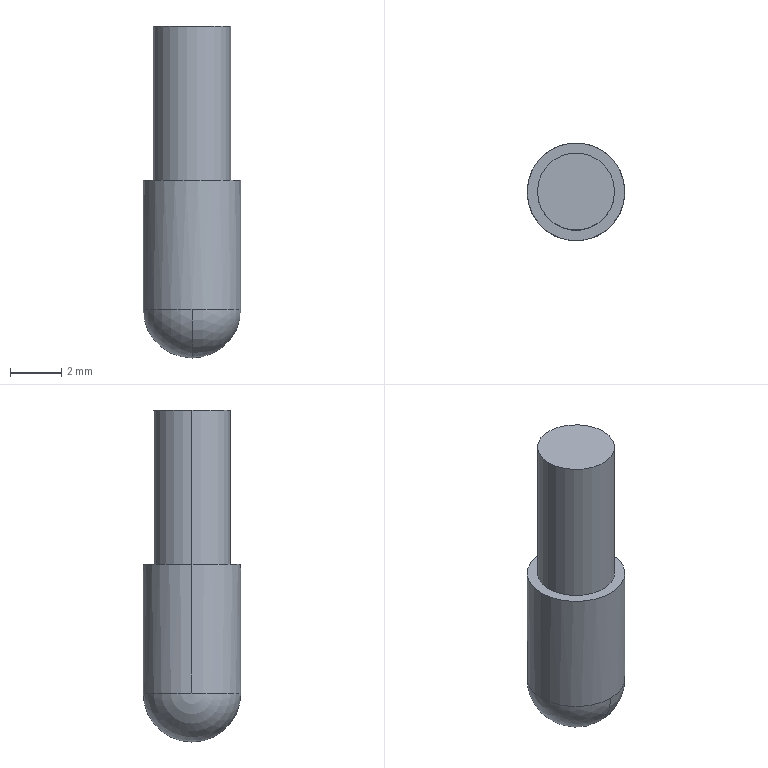Part | STEP file | CKFQAGG3-P3.8-L6-B5_Default | 1 solid | 8 faces | box 3.8 x 3.8 x 12.9 mm | volume 113.483 mm3 | cylinder 4 | sphere 2 | plane 2 | commonest cylinder face diameters 3 x2 3.8 x2
STEP:
#1=CARTESIAN_POINT('',(0.,0.,0.));
#2=DIRECTION('',(0.,0.,1.));
#3=DIRECTION('',(1.,0.,0.));
#4=AXIS2_PLACEMENT_3D('',#1,#2,#3);
#5=CARTESIAN_POINT('',(-1.5,0.,12.9));
#6=VERTEX_POINT('',#5);
#7=CARTESIAN_POINT('',(1.5,0.,12.9));
#8=VERTEX_POINT('',#7);
#9=CARTESIAN_POINT('',(0.,0.,12.9));
#10=DIRECTION('',(0.,0.,-1.));
#11=DIRECTION('',(-1.,0.,0.));
#12=AXIS2_PLACEMENT_3D('',#9,#10,#11);
#13=CIRCLE('',#12,1.5);
#14=CARTESIAN_POINT('',(0.,0.,0.));
#15=DIRECTION('',(0.,0.,-1.));
#16=DIRECTION('',(-1.,0.,0.));
#17=AXIS2_PLACEMENT_3D('',#14,#15,#16);
#18=CYLINDRICAL_SURFACE('',#17,1.5);
#19=CARTESIAN_POINT('',(0.,-12.9));
#20=DIRECTION('',(1.,0.));
#21=VECTOR('',#20,1.);
#22=LINE('',#19,#21);
#23=(GEOMETRIC_REPRESENTATION_CONTEXT(2)PARAMETRIC_REPRESENTATION_CONTEXT()REPRESENTATION_CONTEXT('',''));
#24=DEFINITIONAL_REPRESENTATION('',(#22),#23);
#25=PCURVE('',#18,#24);
#26=CARTESIAN_POINT('',(0.,1.5,12.9));
#27=DIRECTION('',(0.,0.,1.));
#28=DIRECTION('',(1.,0.,0.));
#29=AXIS2_PLACEMENT_3D('',#26,#27,#28);
#30=PLANE('',#29);
#31=CARTESIAN_POINT('',(-1.5,-1.5));
#32=CARTESIAN_POINT('',(-1.5,1.098));
#33=CARTESIAN_POINT('',(0.75,-0.201));
#34=CARTESIAN_POINT('',(3.,-1.5));
#35=CARTESIAN_POINT('',(0.75,-2.799));
#36=CARTESIAN_POINT('',(-1.5,-4.098));
#37=CARTESIAN_POINT('',(-1.5,-1.5));
#38=(BOUNDED_CURVE()B_SPLINE_CURVE(2,(#31,#32,#33,#34,#35,#36,#37),.UNSPECIFIED.,.T.,.F.)B_SPLINE_CURVE_WITH_KNOTS((1,2,2,2,2,1),(-2.094,0.,2.094,4.189,6.283,8.378),.UNSPECIFIED.)CURVE()GEOMETRIC_REPRESENTATION_ITEM()RATIONAL_B_SPLINE_CURVE((1.,0.5,1.,0.5,1.,0.5,1.))REPRESENTATION_ITEM(''));
#39=(GEOMETRIC_REPRESENTATION_CONTEXT(2)PARAMETRIC_REPRESENTATION_CONTEXT()REPRESENTATION_CONTEXT('',''));
#40=DEFINITIONAL_REPRESENTATION('',(#38),#39);
#41=PCURVE('',#30,#40);
#42=SURFACE_CURVE('',#13,(#25,#41),.PCURVE_S1.);
#43=EDGE_CURVE('',#6,#8,#42,.T.);
#44=ORIENTED_EDGE('',*,*,#43,.T.);
#45=CARTESIAN_POINT('',(1.5,0.,6.9));
#46=VERTEX_POINT('',#45);
#47=CARTESIAN_POINT('',(1.5,0.,0.));
#48=DIRECTION('',(0.,0.,-1.));
#49=VECTOR('',#48,1.);
#50=LINE('',#47,#49);
#51=CARTESIAN_POINT('',(3.142,0.));
#52=DIRECTION('',(0.,1.));
#53=VECTOR('',#52,1.);
#54=LINE('',#51,#53);
#55=(GEOMETRIC_REPRESENTATION_CONTEXT(2)PARAMETRIC_REPRESENTATION_CONTEXT()REPRESENTATION_CONTEXT('',''));
#56=DEFINITIONAL_REPRESENTATION('',(#54),#55);
#57=PCURVE('',#18,#56);
#58=CARTESIAN_POINT('',(0.,0.,0.));
#59=DIRECTION('',(0.,0.,-1.));
#60=DIRECTION('',(-1.,0.,0.));
#61=AXIS2_PLACEMENT_3D('',#58,#59,#60);
#62=CYLINDRICAL_SURFACE('',#61,1.5);
#63=CARTESIAN_POINT('',(3.142,0.));
#64=DIRECTION('',(0.,1.));
#65=VECTOR('',#64,1.);
#66=LINE('',#63,#65);
#67=(GEOMETRIC_REPRESENTATION_CONTEXT(2)PARAMETRIC_REPRESENTATION_CONTEXT()REPRESENTATION_CONTEXT('',''));
#68=DEFINITIONAL_REPRESENTATION('',(#66),#67);
#69=PCURVE('',#62,#68);
#70=SURFACE_CURVE('',#50,(#57,#69),.PCURVE_S1.);
#71=EDGE_CURVE('',#8,#46,#70,.T.);
#72=ORIENTED_EDGE('',*,*,#71,.T.);
#73=CARTESIAN_POINT('',(-1.5,0.,6.9));
#74=VERTEX_POINT('',#73);
#75=CARTESIAN_POINT('',(0.,0.,6.9));
#76=DIRECTION('',(0.,0.,-1.));
#77=DIRECTION('',(-1.,0.,0.));
#78=AXIS2_PLACEMENT_3D('',#75,#76,#77);
#79=CIRCLE('',#78,1.5);
#80=CARTESIAN_POINT('',(0.,-6.9));
#81=DIRECTION('',(1.,0.));
#82=VECTOR('',#81,1.);
#83=LINE('',#80,#82);
#84=(GEOMETRIC_REPRESENTATION_CONTEXT(2)PARAMETRIC_REPRESENTATION_CONTEXT()REPRESENTATION_CONTEXT('',''));
#85=DEFINITIONAL_REPRESENTATION('',(#83),#84);
#86=PCURVE('',#18,#85);
#87=CARTESIAN_POINT('',(0.,1.9,6.9));
#88=DIRECTION('',(0.,0.,1.));
#89=DIRECTION('',(1.,0.,0.));
#90=AXIS2_PLACEMENT_3D('',#87,#88,#89);
#91=PLANE('',#90);
#92=CARTESIAN_POINT('',(-1.5,-1.9));
#93=CARTESIAN_POINT('',(-1.5,0.6981));
#94=CARTESIAN_POINT('',(0.75,-0.601));
#95=CARTESIAN_POINT('',(3.,-1.9));
#96=CARTESIAN_POINT('',(0.75,-3.199));
#97=CARTESIAN_POINT('',(-1.5,-4.498));
#98=CARTESIAN_POINT('',(-1.5,-1.9));
#99=(BOUNDED_CURVE()B_SPLINE_CURVE(2,(#92,#93,#94,#95,#96,#97,#98),.UNSPECIFIED.,.T.,.F.)B_SPLINE_CURVE_WITH_KNOTS((1,2,2,2,2,1),(-2.094,0.,2.094,4.189,6.283,8.378),.UNSPECIFIED.)CURVE()GEOMETRIC_REPRESENTATION_ITEM()RATIONAL_B_SPLINE_CURVE((1.,0.5,1.,0.5,1.,0.5,1.))REPRESENTATION_ITEM(''));
#100=(GEOMETRIC_REPRESENTATION_CONTEXT(2)PARAMETRIC_REPRESENTATION_CONTEXT()REPRESENTATION_CONTEXT('',''));
#101=DEFINITIONAL_REPRESENTATION('',(#99),#100);
#102=PCURVE('',#91,#101);
#103=SURFACE_CURVE('',#79,(#86,#102),.PCURVE_S1.);
#104=EDGE_CURVE('',#74,#46,#103,.T.);
#105=ORIENTED_EDGE('',*,*,#104,.F.);
#106=CARTESIAN_POINT('',(-1.5,0.,0.));
#107=DIRECTION('',(0.,0.,-1.));
#108=VECTOR('',#107,1.);
#109=LINE('',#106,#108);
#110=CARTESIAN_POINT('',(0.,0.));
#111=DIRECTION('',(0.,1.));
#112=VECTOR('',#111,1.);
#113=LINE('',#110,#112);
#114=(GEOMETRIC_REPRESENTATION_CONTEXT(2)PARAMETRIC_REPRESENTATION_CONTEXT()REPRESENTATION_CONTEXT('',''));
#115=DEFINITIONAL_REPRESENTATION('',(#113),#114);
#116=PCURVE('',#18,#115);
#117=CARTESIAN_POINT('',(6.283,0.));
#118=DIRECTION('',(0.,1.));
#119=VECTOR('',#118,1.);
#120=LINE('',#117,#119);
#121=(GEOMETRIC_REPRESENTATION_CONTEXT(2)PARAMETRIC_REPRESENTATION_CONTEXT()REPRESENTATION_CONTEXT('',''));
#122=DEFINITIONAL_REPRESENTATION('',(#120),#121);
#123=PCURVE('',#62,#122);
#124=SURFACE_CURVE('',#109,(#116,#123),.PCURVE_S1.);
#125=EDGE_CURVE('',#6,#74,#124,.T.);
#126=ORIENTED_EDGE('',*,*,#125,.F.);
#127=EDGE_LOOP('',(#44,#72,#105,#126));
#128=FACE_BOUND('',#127,.T.);
#129=ADVANCED_FACE('',(#128),#18,.T.);
#130=CARTESIAN_POINT('',(-1.9,0.,6.9));
#131=VERTEX_POINT('',#130);
#132=CARTESIAN_POINT('',(1.9,0.,6.9));
#133=VERTEX_POINT('',#132);
#134=CARTESIAN_POINT('',(0.,0.,6.9));
#135=DIRECTION('',(0.,0.,-1.));
#136=DIRECTION('',(-1.,0.,0.));
#137=AXIS2_PLACEMENT_3D('',#134,#135,#136);
#138=CIRCLE('',#137,1.9);
#139=CARTESIAN_POINT('',(0.,0.,0.));
#140=DIRECTION('',(0.,0.,-1.));
#141=DIRECTION('',(-1.,0.,0.));
#142=AXIS2_PLACEMENT_3D('',#139,#140,#141);
#143=CYLINDRICAL_SURFACE('',#142,1.9);
#144=CARTESIAN_POINT('',(0.,-6.9));
#145=DIRECTION('',(1.,0.));
#146=VECTOR('',#145,1.);
#147=LINE('',#144,#146);
#148=(GEOMETRIC_REPRESENTATION_CONTEXT(2)PARAMETRIC_REPRESENTATION_CONTEXT()REPRESENTATION_CONTEXT('',''));
#149=DEFINITIONAL_REPRESENTATION('',(#147),#148);
#150=PCURVE('',#143,#149);
#151=CARTESIAN_POINT('',(-1.9,-1.9));
#152=CARTESIAN_POINT('',(-1.9,1.391));
#153=CARTESIAN_POINT('',(0.95,-0.2546));
#154=CARTESIAN_POINT('',(3.8,-1.9));
#155=CARTESIAN_POINT('',(0.95,-3.545));
#156=CARTESIAN_POINT('',(-1.9,-5.191));
#157=CARTESIAN_POINT('',(-1.9,-1.9));
#158=(BOUNDED_CURVE()B_SPLINE_CURVE(2,(#151,#152,#153,#154,#155,#156,#157),.UNSPECIFIED.,.T.,.F.)B_SPLINE_CURVE_WITH_KNOTS((1,2,2,2,2,1),(-2.094,0.,2.094,4.189,6.283,8.378),.UNSPECIFIED.)CURVE()GEOMETRIC_REPRESENTATION_ITEM()RATIONAL_B_SPLINE_CURVE((1.,0.5,1.,0.5,1.,0.5,1.))REPRESENTATION_ITEM(''));
#159=(GEOMETRIC_REPRESENTATION_CONTEXT(2)PARAMETRIC_REPRESENTATION_CONTEXT()REPRESENTATION_CONTEXT('',''));
#160=DEFINITIONAL_REPRESENTATION('',(#158),#159);
#161=PCURVE('',#91,#160);
#162=SURFACE_CURVE('',#138,(#150,#161),.PCURVE_S1.);
#163=EDGE_CURVE('',#131,#133,#162,.T.);
#164=ORIENTED_EDGE('',*,*,#163,.T.);
#165=CARTESIAN_POINT('',(1.9,0.,1.9));
#166=VERTEX_POINT('',#165);
#167=CARTESIAN_POINT('',(1.9,0.,0.));
#168=DIRECTION('',(0.,0.,-1.));
#169=VECTOR('',#168,1.);
#170=LINE('',#167,#169);
#171=CARTESIAN_POINT('',(3.142,0.));
#172=DIRECTION('',(0.,1.));
#173=VECTOR('',#172,1.);
#174=LINE('',#171,#173);
#175=(GEOMETRIC_REPRESENTATION_CONTEXT(2)PARAMETRIC_REPRESENTATION_CONTEXT()REPRESENTATION_CONTEXT('',''));
#176=DEFINITIONAL_REPRESENTATION('',(#174),#175);
#177=PCURVE('',#143,#176);
#178=CARTESIAN_POINT('',(0.,0.,0.));
#179=DIRECTION('',(0.,0.,-1.));
#180=DIRECTION('',(-1.,0.,0.));
#181=AXIS2_PLACEMENT_3D('',#178,#179,#180);
#182=CYLINDRICAL_SURFACE('',#181,1.9);
#183=CARTESIAN_POINT('',(3.142,0.));
#184=DIRECTION('',(0.,1.));
#185=VECTOR('',#184,1.);
#186=LINE('',#183,#185);
#187=(GEOMETRIC_REPRESENTATION_CONTEXT(2)PARAMETRIC_REPRESENTATION_CONTEXT()REPRESENTATION_CONTEXT('',''));
#188=DEFINITIONAL_REPRESENTATION('',(#186),#187);
#189=PCURVE('',#182,#188);
#190=SURFACE_CURVE('',#170,(#177,#189),.PCURVE_S1.);
#191=EDGE_CURVE('',#133,#166,#190,.T.);
#192=ORIENTED_EDGE('',*,*,#191,.T.);
#193=CARTESIAN_POINT('',(0.,1.9,1.9));
#194=VERTEX_POINT('',#193);
#195=CARTESIAN_POINT('',(0.,0.,1.9));
#196=DIRECTION('',(0.,0.,-1.));
#197=DIRECTION('',(-1.,0.,0.));
#198=AXIS2_PLACEMENT_3D('',#195,#196,#197);
#199=CIRCLE('',#198,1.9);
#200=CARTESIAN_POINT('',(0.,-1.9));
#201=DIRECTION('',(1.,0.));
#202=VECTOR('',#201,1.);
#203=LINE('',#200,#202);
#204=(GEOMETRIC_REPRESENTATION_CONTEXT(2)PARAMETRIC_REPRESENTATION_CONTEXT()REPRESENTATION_CONTEXT('',''));
#205=DEFINITIONAL_REPRESENTATION('',(#203),#204);
#206=PCURVE('',#143,#205);
#207=CARTESIAN_POINT('',(0.,0.,1.9));
#208=DIRECTION('',(-1.,0.,0.));
#209=DIRECTION('',(0.,-1.,0.));
#210=AXIS2_PLACEMENT_3D('',#207,#208,#209);
#211=SPHERICAL_SURFACE('',#210,1.9);
#212=CARTESIAN_POINT('',(3.142,1.571));
#213=DIRECTION('',(0.,-1.));
#214=VECTOR('',#213,1.);
#215=LINE('',#212,#214);
#216=(GEOMETRIC_REPRESENTATION_CONTEXT(2)PARAMETRIC_REPRESENTATION_CONTEXT()REPRESENTATION_CONTEXT('',''));
#217=DEFINITIONAL_REPRESENTATION('',(#215),#216);
#218=PCURVE('',#211,#217);
#219=SURFACE_CURVE('',#199,(#206,#218),.PCURVE_S1.);
#220=EDGE_CURVE('',#194,#166,#219,.T.);
#221=ORIENTED_EDGE('',*,*,#220,.F.);
#222=CARTESIAN_POINT('',(-1.9,0.,1.9));
#223=VERTEX_POINT('',#222);
#224=CARTESIAN_POINT('',(0.,0.,1.9));
#225=DIRECTION('',(0.,0.,-1.));
#226=DIRECTION('',(-1.,0.,0.));
#227=AXIS2_PLACEMENT_3D('',#224,#225,#226);
#228=CIRCLE('',#227,1.9);
#229=CARTESIAN_POINT('',(0.,-1.9));
#230=DIRECTION('',(1.,0.));
#231=VECTOR('',#230,1.);
#232=LINE('',#229,#231);
#233=(GEOMETRIC_REPRESENTATION_CONTEXT(2)PARAMETRIC_REPRESENTATION_CONTEXT()REPRESENTATION_CONTEXT('',''));
#234=DEFINITIONAL_REPRESENTATION('',(#232),#233);
#235=PCURVE('',#143,#234);
#236=CARTESIAN_POINT('',(0.,0.,1.9));
#237=DIRECTION('',(-1.,0.,0.));
#238=DIRECTION('',(0.,-1.,0.));
#239=AXIS2_PLACEMENT_3D('',#236,#237,#238);
#240=SPHERICAL_SURFACE('',#239,1.9);
#241=CARTESIAN_POINT('',(3.142,1.571));
#242=CARTESIAN_POINT('',(3.142,1.547));
#243=CARTESIAN_POINT('',(3.142,1.499));
#244=CARTESIAN_POINT('',(3.142,1.428));
#245=CARTESIAN_POINT('',(3.142,1.357));
#246=CARTESIAN_POINT('',(3.142,1.285));
#247=CARTESIAN_POINT('',(3.142,1.214));
#248=CARTESIAN_POINT('',(3.142,1.142));
#249=CARTESIAN_POINT('',(3.142,1.071));
#250=CARTESIAN_POINT('',(3.142,0.9996));
#251=CARTESIAN_POINT('',(3.142,0.9282));
#252=CARTESIAN_POINT('',(3.142,0.8568));
#253=CARTESIAN_POINT('',(3.142,0.7854));
#254=CARTESIAN_POINT('',(3.142,0.714));
#255=CARTESIAN_POINT('',(3.142,0.6426));
#256=CARTESIAN_POINT('',(3.142,0.5712));
#257=CARTESIAN_POINT('',(3.142,0.4998));
#258=CARTESIAN_POINT('',(3.142,0.4284));
#259=CARTESIAN_POINT('',(3.142,0.357));
#260=CARTESIAN_POINT('',(3.142,0.2856));
#261=CARTESIAN_POINT('',(3.142,0.2142));
#262=CARTESIAN_POINT('',(3.142,0.1428));
#263=CARTESIAN_POINT('',(3.142,0.0714));
#264=CARTESIAN_POINT('',(3.142,0.0238));
#265=CARTESIAN_POINT('',(3.142,0.));
#266=B_SPLINE_CURVE_WITH_KNOTS('',3,(#241,#242,#243,#244,#245,#246,#247,#248,#249,#250,#251,#252,#253,#254,#255,#256,#257,#258,#259,#260,#261,#262,#263,#264,#265),.UNSPECIFIED.,.F.,.F.,(4,1,1,1,1,1,1,1,1,1,1,1,1,1,1,1,1,1,1,1,1,1,4),(0.,0.0714,0.1428,0.2142,0.2856,0.357,0.4284,0.4998,0.5712,0.6426,0.714,0.7854,0.8568,0.9282,0.9996,1.071,1.142,1.214,1.285,1.357,1.428,1.499,1.571),.QUASI_UNIFORM_KNOTS.);
#267=(GEOMETRIC_REPRESENTATION_CONTEXT(2)PARAMETRIC_REPRESENTATION_CONTEXT()REPRESENTATION_CONTEXT('',''));
#268=DEFINITIONAL_REPRESENTATION('',(#266),#267);
#269=PCURVE('',#240,#268);
#270=SURFACE_CURVE('',#228,(#235,#269),.PCURVE_S1.);
#271=EDGE_CURVE('',#223,#194,#270,.T.);
#272=ORIENTED_EDGE('',*,*,#271,.F.);
#273=CARTESIAN_POINT('',(-1.9,0.,0.));
#274=DIRECTION('',(0.,0.,-1.));
#275=VECTOR('',#274,1.);
#276=LINE('',#273,#275);
#277=CARTESIAN_POINT('',(0.,0.));
#278=DIRECTION('',(0.,1.));
#279=VECTOR('',#278,1.);
#280=LINE('',#277,#279);
#281=(GEOMETRIC_REPRESENTATION_CONTEXT(2)PARAMETRIC_REPRESENTATION_CONTEXT()REPRESENTATION_CONTEXT('',''));
#282=DEFINITIONAL_REPRESENTATION('',(#280),#281);
#283=PCURVE('',#143,#282);
#284=CARTESIAN_POINT('',(6.283,0.));
#285=DIRECTION('',(0.,1.));
#286=VECTOR('',#285,1.);
#287=LINE('',#284,#286);
#288=(GEOMETRIC_REPRESENTATION_CONTEXT(2)PARAMETRIC_REPRESENTATION_CONTEXT()REPRESENTATION_CONTEXT('',''));
#289=DEFINITIONAL_REPRESENTATION('',(#287),#288);
#290=PCURVE('',#182,#289);
#291=SURFACE_CURVE('',#276,(#283,#290),.PCURVE_S1.);
#292=EDGE_CURVE('',#131,#223,#291,.T.);
#293=ORIENTED_EDGE('',*,*,#292,.F.);
#294=EDGE_LOOP('',(#164,#192,#221,#272,#293));
#295=FACE_BOUND('',#294,.T.);
#296=ADVANCED_FACE('',(#295),#143,.T.);
#297=CARTESIAN_POINT('',(0.,-1.9,1.9));
#298=VERTEX_POINT('',#297);
#299=CARTESIAN_POINT('',(0.,0.,1.9));
#300=DIRECTION('',(0.,0.,-1.));
#301=DIRECTION('',(-1.,0.,0.));
#302=AXIS2_PLACEMENT_3D('',#299,#300,#301);
#303=CIRCLE('',#302,1.9);
#304=CARTESIAN_POINT('',(6.283,-4.712));
#305=DIRECTION('',(0.,1.));
#306=VECTOR('',#305,1.);
#307=LINE('',#304,#306);
#308=(GEOMETRIC_REPRESENTATION_CONTEXT(2)PARAMETRIC_REPRESENTATION_CONTEXT()REPRESENTATION_CONTEXT('',''));
#309=DEFINITIONAL_REPRESENTATION('',(#307),#308);
#310=PCURVE('',#240,#309);
#311=CARTESIAN_POINT('',(0.,-1.9));
#312=DIRECTION('',(1.,0.));
#313=VECTOR('',#312,1.);
#314=LINE('',#311,#313);
#315=(GEOMETRIC_REPRESENTATION_CONTEXT(2)PARAMETRIC_REPRESENTATION_CONTEXT()REPRESENTATION_CONTEXT('',''));
#316=DEFINITIONAL_REPRESENTATION('',(#314),#315);
#317=PCURVE('',#182,#316);
#318=SURFACE_CURVE('',#303,(#310,#317),.PCURVE_S1.);
#319=EDGE_CURVE('',#298,#223,#318,.T.);
#320=ORIENTED_EDGE('',*,*,#319,.T.);
#321=ORIENTED_EDGE('',*,*,#271,.T.);
#322=CARTESIAN_POINT('',(0.,0.,0.));
#323=VERTEX_POINT('',#322);
#324=CARTESIAN_POINT('',(0.,0.,1.9));
#325=DIRECTION('',(-1.,0.,0.));
#326=DIRECTION('',(0.,-1.,0.));
#327=AXIS2_PLACEMENT_3D('',#324,#325,#326);
#328=CIRCLE('',#327,1.9);
#329=CARTESIAN_POINT('',(0.,0.));
#330=DIRECTION('',(1.,0.));
#331=VECTOR('',#330,1.);
#332=LINE('',#329,#331);
#333=(GEOMETRIC_REPRESENTATION_CONTEXT(2)PARAMETRIC_REPRESENTATION_CONTEXT()REPRESENTATION_CONTEXT('',''));
#334=DEFINITIONAL_REPRESENTATION('',(#332),#333);
#335=PCURVE('',#240,#334);
#336=CARTESIAN_POINT('',(0.,0.));
#337=DIRECTION('',(1.,0.));
#338=VECTOR('',#337,1.);
#339=LINE('',#336,#338);
#340=(GEOMETRIC_REPRESENTATION_CONTEXT(2)PARAMETRIC_REPRESENTATION_CONTEXT()REPRESENTATION_CONTEXT('',''));
#341=DEFINITIONAL_REPRESENTATION('',(#339),#340);
#342=PCURVE('',#211,#341);
#343=SURFACE_CURVE('',#328,(#335,#342),.PCURVE_S1.);
#344=EDGE_CURVE('',#194,#323,#343,.T.);
#345=ORIENTED_EDGE('',*,*,#344,.T.);
#346=CARTESIAN_POINT('',(0.,0.,1.9));
#347=DIRECTION('',(1.,0.,0.));
#348=DIRECTION('',(0.,0.,-1.));
#349=AXIS2_PLACEMENT_3D('',#346,#347,#348);
#350=CIRCLE('',#349,1.9);
#351=CARTESIAN_POINT('',(6.283,0.));
#352=CARTESIAN_POINT('',(6.259,0.));
#353=CARTESIAN_POINT('',(6.212,0.));
#354=CARTESIAN_POINT('',(6.14,0.));
#355=CARTESIAN_POINT('',(6.069,0.));
#356=CARTESIAN_POINT('',(5.998,0.));
#357=CARTESIAN_POINT('',(5.926,0.));
#358=CARTESIAN_POINT('',(5.855,0.));
#359=CARTESIAN_POINT('',(5.783,0.));
#360=CARTESIAN_POINT('',(5.712,0.));
#361=CARTESIAN_POINT('',(5.641,0.));
#362=CARTESIAN_POINT('',(5.569,0.));
#363=CARTESIAN_POINT('',(5.498,0.));
#364=CARTESIAN_POINT('',(5.426,0.));
#365=CARTESIAN_POINT('',(5.355,0.));
#366=CARTESIAN_POINT('',(5.284,0.));
#367=CARTESIAN_POINT('',(5.212,0.));
#368=CARTESIAN_POINT('',(5.141,0.));
#369=CARTESIAN_POINT('',(5.069,0.));
#370=CARTESIAN_POINT('',(4.998,0.));
#371=CARTESIAN_POINT('',(4.927,0.));
#372=CARTESIAN_POINT('',(4.855,0.));
#373=CARTESIAN_POINT('',(4.784,0.));
#374=CARTESIAN_POINT('',(4.736,0.));
#375=CARTESIAN_POINT('',(4.712,0.));
#376=B_SPLINE_CURVE_WITH_KNOTS('',3,(#351,#352,#353,#354,#355,#356,#357,#358,#359,#360,#361,#362,#363,#364,#365,#366,#367,#368,#369,#370,#371,#372,#373,#374,#375),.UNSPECIFIED.,.F.,.F.,(4,1,1,1,1,1,1,1,1,1,1,1,1,1,1,1,1,1,1,1,1,1,4),(4.712,4.784,4.855,4.927,4.998,5.069,5.141,5.212,5.284,5.355,5.426,5.498,5.569,5.641,5.712,5.783,5.855,5.926,5.998,6.069,6.14,6.212,6.283),.QUASI_UNIFORM_KNOTS.);
#377=(GEOMETRIC_REPRESENTATION_CONTEXT(2)PARAMETRIC_REPRESENTATION_CONTEXT()REPRESENTATION_CONTEXT('',''));
#378=DEFINITIONAL_REPRESENTATION('',(#376),#377);
#379=PCURVE('',#240,#378);
#380=CARTESIAN_POINT('',(6.283,0.));
#381=CARTESIAN_POINT('',(6.259,0.));
#382=CARTESIAN_POINT('',(6.212,0.));
#383=CARTESIAN_POINT('',(6.14,0.));
#384=CARTESIAN_POINT('',(6.069,0.));
#385=CARTESIAN_POINT('',(5.998,0.));
#386=CARTESIAN_POINT('',(5.926,0.));
#387=CARTESIAN_POINT('',(5.855,0.));
#388=CARTESIAN_POINT('',(5.783,0.));
#389=CARTESIAN_POINT('',(5.712,0.));
#390=CARTESIAN_POINT('',(5.641,0.));
#391=CARTESIAN_POINT('',(5.569,0.));
#392=CARTESIAN_POINT('',(5.498,0.));
#393=CARTESIAN_POINT('',(5.426,0.));
#394=CARTESIAN_POINT('',(5.355,0.));
#395=CARTESIAN_POINT('',(5.284,0.));
#396=CARTESIAN_POINT('',(5.212,0.));
#397=CARTESIAN_POINT('',(5.141,0.));
#398=CARTESIAN_POINT('',(5.069,0.));
#399=CARTESIAN_POINT('',(4.998,0.));
#400=CARTESIAN_POINT('',(4.927,0.));
#401=CARTESIAN_POINT('',(4.855,0.));
#402=CARTESIAN_POINT('',(4.784,0.));
#403=CARTESIAN_POINT('',(4.736,0.));
#404=CARTESIAN_POINT('',(4.712,0.));
#405=B_SPLINE_CURVE_WITH_KNOTS('',3,(#380,#381,#382,#383,#384,#385,#386,#387,#388,#389,#390,#391,#392,#393,#394,#395,#396,#397,#398,#399,#400,#401,#402,#403,#404),.UNSPECIFIED.,.F.,.F.,(4,1,1,1,1,1,1,1,1,1,1,1,1,1,1,1,1,1,1,1,1,1,4),(4.712,4.784,4.855,4.927,4.998,5.069,5.141,5.212,5.284,5.355,5.426,5.498,5.569,5.641,5.712,5.783,5.855,5.926,5.998,6.069,6.14,6.212,6.283),.QUASI_UNIFORM_KNOTS.);
#406=(GEOMETRIC_REPRESENTATION_CONTEXT(2)PARAMETRIC_REPRESENTATION_CONTEXT()REPRESENTATION_CONTEXT('',''));
#407=DEFINITIONAL_REPRESENTATION('',(#405),#406);
#408=PCURVE('',#211,#407);
#409=SURFACE_CURVE('',#350,(#379,#408),.PCURVE_S1.);
#410=EDGE_CURVE('',#298,#323,#409,.T.);
#411=ORIENTED_EDGE('',*,*,#410,.F.);
#412=EDGE_LOOP('',(#320,#321,#345,#411));
#413=FACE_BOUND('',#412,.T.);
#414=ADVANCED_FACE('',(#413),#240,.T.);
#415=ORIENTED_EDGE('',*,*,#344,.F.);
#416=ORIENTED_EDGE('',*,*,#220,.T.);
#417=CARTESIAN_POINT('',(0.,0.,1.9));
#418=DIRECTION('',(0.,0.,-1.));
#419=DIRECTION('',(-1.,0.,0.));
#420=AXIS2_PLACEMENT_3D('',#417,#418,#419);
#421=CIRCLE('',#420,1.9);
#422=CARTESIAN_POINT('',(6.283,-1.571));
#423=CARTESIAN_POINT('',(6.283,-1.547));
#424=CARTESIAN_POINT('',(6.283,-1.499));
#425=CARTESIAN_POINT('',(6.283,-1.428));
#426=CARTESIAN_POINT('',(6.283,-1.357));
#427=CARTESIAN_POINT('',(6.283,-1.285));
#428=CARTESIAN_POINT('',(6.283,-1.214));
#429=CARTESIAN_POINT('',(6.283,-1.142));
#430=CARTESIAN_POINT('',(6.283,-1.071));
#431=CARTESIAN_POINT('',(6.283,-0.9996));
#432=CARTESIAN_POINT('',(6.283,-0.9282));
#433=CARTESIAN_POINT('',(6.283,-0.8568));
#434=CARTESIAN_POINT('',(6.283,-0.7854));
#435=CARTESIAN_POINT('',(6.283,-0.714));
#436=CARTESIAN_POINT('',(6.283,-0.6426));
#437=CARTESIAN_POINT('',(6.283,-0.5712));
#438=CARTESIAN_POINT('',(6.283,-0.4998));
#439=CARTESIAN_POINT('',(6.283,-0.4284));
#440=CARTESIAN_POINT('',(6.283,-0.357));
#441=CARTESIAN_POINT('',(6.283,-0.2856));
#442=CARTESIAN_POINT('',(6.283,-0.2142));
#443=CARTESIAN_POINT('',(6.283,-0.1428));
#444=CARTESIAN_POINT('',(6.283,-0.0714));
#445=CARTESIAN_POINT('',(6.283,-0.0238));
#446=CARTESIAN_POINT('',(6.283,0.));
#447=B_SPLINE_CURVE_WITH_KNOTS('',3,(#422,#423,#424,#425,#426,#427,#428,#429,#430,#431,#432,#433,#434,#435,#436,#437,#438,#439,#440,#441,#442,#443,#444,#445,#446),.UNSPECIFIED.,.F.,.F.,(4,1,1,1,1,1,1,1,1,1,1,1,1,1,1,1,1,1,1,1,1,1,4),(3.142,3.213,3.284,3.356,3.427,3.499,3.57,3.641,3.713,3.784,3.856,3.927,3.998,4.07,4.141,4.213,4.284,4.355,4.427,4.498,4.57,4.641,4.712),.QUASI_UNIFORM_KNOTS.);
#448=(GEOMETRIC_REPRESENTATION_CONTEXT(2)PARAMETRIC_REPRESENTATION_CONTEXT()REPRESENTATION_CONTEXT('',''));
#449=DEFINITIONAL_REPRESENTATION('',(#447),#448);
#450=PCURVE('',#211,#449);
#451=CARTESIAN_POINT('',(0.,-1.9));
#452=DIRECTION('',(1.,0.));
#453=VECTOR('',#452,1.);
#454=LINE('',#451,#453);
#455=(GEOMETRIC_REPRESENTATION_CONTEXT(2)PARAMETRIC_REPRESENTATION_CONTEXT()REPRESENTATION_CONTEXT('',''));
#456=DEFINITIONAL_REPRESENTATION('',(#454),#455);
#457=PCURVE('',#182,#456);
#458=SURFACE_CURVE('',#421,(#450,#457),.PCURVE_S1.);
#459=EDGE_CURVE('',#166,#298,#458,.T.);
#460=ORIENTED_EDGE('',*,*,#459,.T.);
#461=ORIENTED_EDGE('',*,*,#410,.T.);
#462=EDGE_LOOP('',(#415,#416,#460,#461));
#463=FACE_BOUND('',#462,.T.);
#464=ADVANCED_FACE('',(#463),#211,.T.);
#465=ORIENTED_EDGE('',*,*,#191,.F.);
#466=CARTESIAN_POINT('',(0.,0.,6.9));
#467=DIRECTION('',(0.,0.,-1.));
#468=DIRECTION('',(-1.,0.,0.));
#469=AXIS2_PLACEMENT_3D('',#466,#467,#468);
#470=CIRCLE('',#469,1.9);
#471=CARTESIAN_POINT('',(0.,-6.9));
#472=DIRECTION('',(1.,0.));
#473=VECTOR('',#472,1.);
#474=LINE('',#471,#473);
#475=(GEOMETRIC_REPRESENTATION_CONTEXT(2)PARAMETRIC_REPRESENTATION_CONTEXT()REPRESENTATION_CONTEXT('',''));
#476=DEFINITIONAL_REPRESENTATION('',(#474),#475);
#477=PCURVE('',#182,#476);
#478=CARTESIAN_POINT('',(-1.9,-1.9));
#479=CARTESIAN_POINT('',(-1.9,1.391));
#480=CARTESIAN_POINT('',(0.95,-0.2546));
#481=CARTESIAN_POINT('',(3.8,-1.9));
#482=CARTESIAN_POINT('',(0.95,-3.545));
#483=CARTESIAN_POINT('',(-1.9,-5.191));
#484=CARTESIAN_POINT('',(-1.9,-1.9));
#485=(BOUNDED_CURVE()B_SPLINE_CURVE(2,(#478,#479,#480,#481,#482,#483,#484),.UNSPECIFIED.,.T.,.F.)B_SPLINE_CURVE_WITH_KNOTS((1,2,2,2,2,1),(-2.094,0.,2.094,4.189,6.283,8.378),.UNSPECIFIED.)CURVE()GEOMETRIC_REPRESENTATION_ITEM()RATIONAL_B_SPLINE_CURVE((1.,0.5,1.,0.5,1.,0.5,1.))REPRESENTATION_ITEM(''));
#486=(GEOMETRIC_REPRESENTATION_CONTEXT(2)PARAMETRIC_REPRESENTATION_CONTEXT()REPRESENTATION_CONTEXT('',''));
#487=DEFINITIONAL_REPRESENTATION('',(#485),#486);
#488=PCURVE('',#91,#487);
#489=SURFACE_CURVE('',#470,(#477,#488),.PCURVE_S1.);
#490=EDGE_CURVE('',#133,#131,#489,.T.);
#491=ORIENTED_EDGE('',*,*,#490,.T.);
#492=ORIENTED_EDGE('',*,*,#292,.T.);
#493=ORIENTED_EDGE('',*,*,#319,.F.);
#494=ORIENTED_EDGE('',*,*,#459,.F.);
#495=EDGE_LOOP('',(#465,#491,#492,#493,#494));
#496=FACE_BOUND('',#495,.T.);
#497=ADVANCED_FACE('',(#496),#182,.T.);
#498=ORIENTED_EDGE('',*,*,#104,.T.);
#499=CARTESIAN_POINT('',(0.,0.,6.9));
#500=DIRECTION('',(0.,0.,-1.));
#501=DIRECTION('',(-1.,0.,0.));
#502=AXIS2_PLACEMENT_3D('',#499,#500,#501);
#503=CIRCLE('',#502,1.5);
#504=CARTESIAN_POINT('',(-1.5,-1.9));
#505=CARTESIAN_POINT('',(-1.5,0.6981));
#506=CARTESIAN_POINT('',(0.75,-0.601));
#507=CARTESIAN_POINT('',(3.,-1.9));
#508=CARTESIAN_POINT('',(0.75,-3.199));
#509=CARTESIAN_POINT('',(-1.5,-4.498));
#510=CARTESIAN_POINT('',(-1.5,-1.9));
#511=(BOUNDED_CURVE()B_SPLINE_CURVE(2,(#504,#505,#506,#507,#508,#509,#510),.UNSPECIFIED.,.T.,.F.)B_SPLINE_CURVE_WITH_KNOTS((1,2,2,2,2,1),(-2.094,0.,2.094,4.189,6.283,8.378),.UNSPECIFIED.)CURVE()GEOMETRIC_REPRESENTATION_ITEM()RATIONAL_B_SPLINE_CURVE((1.,0.5,1.,0.5,1.,0.5,1.))REPRESENTATION_ITEM(''));
#512=(GEOMETRIC_REPRESENTATION_CONTEXT(2)PARAMETRIC_REPRESENTATION_CONTEXT()REPRESENTATION_CONTEXT('',''));
#513=DEFINITIONAL_REPRESENTATION('',(#511),#512);
#514=PCURVE('',#91,#513);
#515=CARTESIAN_POINT('',(0.,-6.9));
#516=DIRECTION('',(1.,0.));
#517=VECTOR('',#516,1.);
#518=LINE('',#515,#517);
#519=(GEOMETRIC_REPRESENTATION_CONTEXT(2)PARAMETRIC_REPRESENTATION_CONTEXT()REPRESENTATION_CONTEXT('',''));
#520=DEFINITIONAL_REPRESENTATION('',(#518),#519);
#521=PCURVE('',#62,#520);
#522=SURFACE_CURVE('',#503,(#514,#521),.PCURVE_S1.);
#523=EDGE_CURVE('',#46,#74,#522,.T.);
#524=ORIENTED_EDGE('',*,*,#523,.T.);
#525=EDGE_LOOP('',(#498,#524));
#526=FACE_BOUND('',#525,.T.);
#527=ORIENTED_EDGE('',*,*,#163,.F.);
#528=ORIENTED_EDGE('',*,*,#490,.F.);
#529=EDGE_LOOP('',(#527,#528));
#530=FACE_BOUND('',#529,.T.);
#531=ADVANCED_FACE('',(#526,#530),#91,.T.);
#532=ORIENTED_EDGE('',*,*,#71,.F.);
#533=CARTESIAN_POINT('',(0.,0.,12.9));
#534=DIRECTION('',(0.,0.,-1.));
#535=DIRECTION('',(-1.,0.,0.));
#536=AXIS2_PLACEMENT_3D('',#533,#534,#535);
#537=CIRCLE('',#536,1.5);
#538=CARTESIAN_POINT('',(0.,-12.9));
#539=DIRECTION('',(1.,0.));
#540=VECTOR('',#539,1.);
#541=LINE('',#538,#540);
#542=(GEOMETRIC_REPRESENTATION_CONTEXT(2)PARAMETRIC_REPRESENTATION_CONTEXT()REPRESENTATION_CONTEXT('',''));
#543=DEFINITIONAL_REPRESENTATION('',(#541),#542);
#544=PCURVE('',#62,#543);
#545=CARTESIAN_POINT('',(-1.5,-1.5));
#546=CARTESIAN_POINT('',(-1.5,1.098));
#547=CARTESIAN_POINT('',(0.75,-0.201));
#548=CARTESIAN_POINT('',(3.,-1.5));
#549=CARTESIAN_POINT('',(0.75,-2.799));
#550=CARTESIAN_POINT('',(-1.5,-4.098));
#551=CARTESIAN_POINT('',(-1.5,-1.5));
#552=(BOUNDED_CURVE()B_SPLINE_CURVE(2,(#545,#546,#547,#548,#549,#550,#551),.UNSPECIFIED.,.T.,.F.)B_SPLINE_CURVE_WITH_KNOTS((1,2,2,2,2,1),(-2.094,0.,2.094,4.189,6.283,8.378),.UNSPECIFIED.)CURVE()GEOMETRIC_REPRESENTATION_ITEM()RATIONAL_B_SPLINE_CURVE((1.,0.5,1.,0.5,1.,0.5,1.))REPRESENTATION_ITEM(''));
#553=(GEOMETRIC_REPRESENTATION_CONTEXT(2)PARAMETRIC_REPRESENTATION_CONTEXT()REPRESENTATION_CONTEXT('',''));
#554=DEFINITIONAL_REPRESENTATION('',(#552),#553);
#555=PCURVE('',#30,#554);
#556=SURFACE_CURVE('',#537,(#544,#555),.PCURVE_S1.);
#557=EDGE_CURVE('',#8,#6,#556,.T.);
#558=ORIENTED_EDGE('',*,*,#557,.T.);
#559=ORIENTED_EDGE('',*,*,#125,.T.);
#560=ORIENTED_EDGE('',*,*,#523,.F.);
#561=EDGE_LOOP('',(#532,#558,#559,#560));
#562=FACE_BOUND('',#561,.T.);
#563=ADVANCED_FACE('',(#562),#62,.T.);
#564=ORIENTED_EDGE('',*,*,#43,.F.);
#565=ORIENTED_EDGE('',*,*,#557,.F.);
#566=EDGE_LOOP('',(#564,#565));
#567=FACE_BOUND('',#566,.T.);
#568=ADVANCED_FACE('',(#567),#30,.T.);
#569=CLOSED_SHELL('',(#129,#296,#414,#464,#497,#531,#563,#568));
#570=MANIFOLD_SOLID_BREP('',#569);
#571=(LENGTH_UNIT()NAMED_UNIT(*)SI_UNIT(.MILLI.,.METRE.));
#572=UNCERTAINTY_MEASURE_WITH_UNIT(LENGTH_MEASURE(0.0000001),#571,'','');
#573=(NAMED_UNIT(*)PLANE_ANGLE_UNIT()SI_UNIT($,.RADIAN.));
#574=(NAMED_UNIT(*)SI_UNIT($,.STERADIAN.)SOLID_ANGLE_UNIT());
#575=(GEOMETRIC_REPRESENTATION_CONTEXT(3)GLOBAL_UNCERTAINTY_ASSIGNED_CONTEXT((#572))GLOBAL_UNIT_ASSIGNED_CONTEXT((#571,#573,#574))REPRESENTATION_CONTEXT('',''));
#576=ADVANCED_BREP_SHAPE_REPRESENTATION('',(#4,#570),#575);